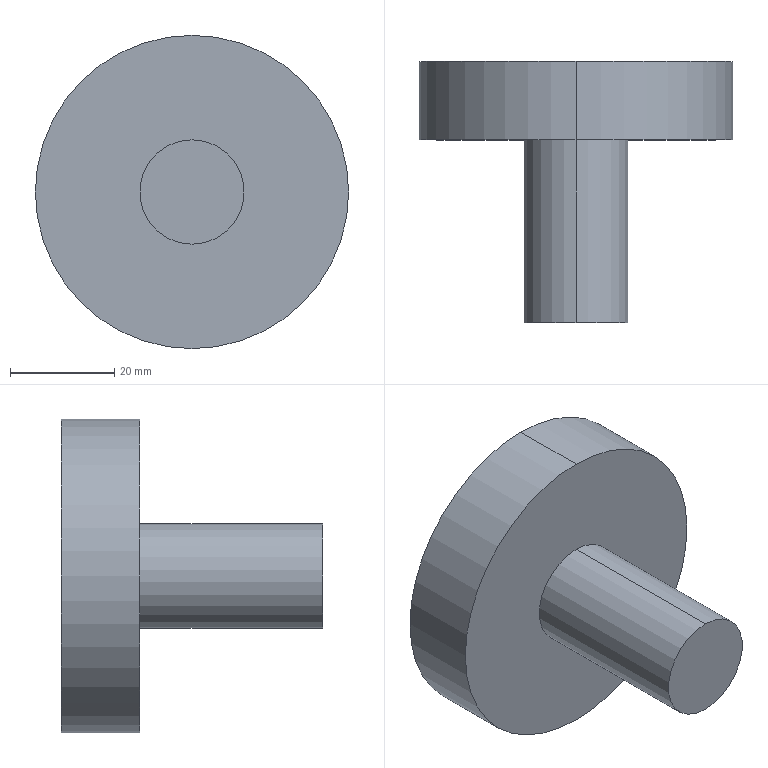Part | STEP file | Part5_1 | 1 solid | 16 faces | box 60 x 50 x 60 mm | volume 49793 mm3 | cylinder 10 | plane 6 | commonest cylinder face diameters 15.4 x2 16.4 x2 18.4 x2 20 x2 60 x2
STEP:
#1=CARTESIAN_POINT('',(0.,0.,0.));
#2=DIRECTION('',(0.,0.,1.));
#3=DIRECTION('',(1.,0.,0.));
#4=AXIS2_PLACEMENT_3D('',#1,#2,#3);
#5=CARTESIAN_POINT('',(0.,84.,-200.8));
#6=VERTEX_POINT('',#5);
#7=CARTESIAN_POINT('',(0.,99.,-200.8));
#8=VERTEX_POINT('',#7);
#9=CARTESIAN_POINT('',(0.,91.5,-200.8));
#10=DIRECTION('',(0.,1.,0.));
#11=VECTOR('',#10,1.);
#12=LINE('',#9,#11);
#13=CARTESIAN_POINT('',(0.,91.5,-210.));
#14=DIRECTION('',(0.,1.,0.));
#15=DIRECTION('',(0.,0.,1.));
#16=AXIS2_PLACEMENT_3D('',#13,#14,#15);
#17=CYLINDRICAL_SURFACE('',#16,9.2);
#18=CARTESIAN_POINT('',(6.283,0.));
#19=DIRECTION('',(0.,1.));
#20=VECTOR('',#19,1.);
#21=LINE('',#18,#20);
#22=(GEOMETRIC_REPRESENTATION_CONTEXT(2)PARAMETRIC_REPRESENTATION_CONTEXT()REPRESENTATION_CONTEXT('',''));
#23=DEFINITIONAL_REPRESENTATION('',(#21),#22);
#24=PCURVE('',#17,#23);
#25=CARTESIAN_POINT('',(0.,91.5,-210.));
#26=DIRECTION('',(0.,1.,0.));
#27=DIRECTION('',(0.,0.,1.));
#28=AXIS2_PLACEMENT_3D('',#25,#26,#27);
#29=CYLINDRICAL_SURFACE('',#28,9.2);
#30=CARTESIAN_POINT('',(0.,0.));
#31=DIRECTION('',(0.,1.));
#32=VECTOR('',#31,1.);
#33=LINE('',#30,#32);
#34=(GEOMETRIC_REPRESENTATION_CONTEXT(2)PARAMETRIC_REPRESENTATION_CONTEXT()REPRESENTATION_CONTEXT('',''));
#35=DEFINITIONAL_REPRESENTATION('',(#33),#34);
#36=PCURVE('',#29,#35);
#37=SURFACE_CURVE('',#12,(#24,#36),.PCURVE_S1.);
#38=EDGE_CURVE('',#6,#8,#37,.T.);
#39=ORIENTED_EDGE('',*,*,#38,.T.);
#40=CARTESIAN_POINT('',(0.,99.,-219.2));
#41=VERTEX_POINT('',#40);
#42=CARTESIAN_POINT('',(0.,99.,-210.));
#43=DIRECTION('',(0.,-1.,0.));
#44=DIRECTION('',(0.,0.,1.));
#45=AXIS2_PLACEMENT_3D('',#42,#43,#44);
#46=CIRCLE('',#45,9.2);
#47=CARTESIAN_POINT('',(6.283,7.5));
#48=DIRECTION('',(-1.,0.));
#49=VECTOR('',#48,1.);
#50=LINE('',#47,#49);
#51=(GEOMETRIC_REPRESENTATION_CONTEXT(2)PARAMETRIC_REPRESENTATION_CONTEXT()REPRESENTATION_CONTEXT('',''));
#52=DEFINITIONAL_REPRESENTATION('',(#50),#51);
#53=PCURVE('',#17,#52);
#54=CARTESIAN_POINT('',(0.,99.,0.));
#55=DIRECTION('',(0.,1.,0.));
#56=DIRECTION('',(0.,0.,1.));
#57=AXIS2_PLACEMENT_3D('',#54,#55,#56);
#58=PLANE('',#57);
#59=CARTESIAN_POINT('',(-200.8,0.));
#60=CARTESIAN_POINT('',(-200.8,-15.935));
#61=CARTESIAN_POINT('',(-214.6,-7.967));
#62=CARTESIAN_POINT('',(-228.4,0.));
#63=CARTESIAN_POINT('',(-214.6,7.967));
#64=CARTESIAN_POINT('',(-200.8,15.935));
#65=CARTESIAN_POINT('',(-200.8,0.));
#66=(BOUNDED_CURVE()B_SPLINE_CURVE(2,(#59,#60,#61,#62,#63,#64,#65),.UNSPECIFIED.,.T.,.F.)B_SPLINE_CURVE_WITH_KNOTS((1,2,2,2,2,1),(-2.094,0.,2.094,4.189,6.283,8.378),.UNSPECIFIED.)CURVE()GEOMETRIC_REPRESENTATION_ITEM()RATIONAL_B_SPLINE_CURVE((1.,0.5,1.,0.5,1.,0.5,1.))REPRESENTATION_ITEM(''));
#67=(GEOMETRIC_REPRESENTATION_CONTEXT(2)PARAMETRIC_REPRESENTATION_CONTEXT()REPRESENTATION_CONTEXT('',''));
#68=DEFINITIONAL_REPRESENTATION('',(#66),#67);
#69=PCURVE('',#58,#68);
#70=SURFACE_CURVE('',#46,(#53,#69),.PCURVE_S1.);
#71=EDGE_CURVE('',#8,#41,#70,.T.);
#72=ORIENTED_EDGE('',*,*,#71,.T.);
#73=CARTESIAN_POINT('',(0.,84.,-219.2));
#74=VERTEX_POINT('',#73);
#75=CARTESIAN_POINT('',(0.,91.5,-219.2));
#76=DIRECTION('',(0.,1.,0.));
#77=VECTOR('',#76,1.);
#78=LINE('',#75,#77);
#79=CARTESIAN_POINT('',(3.142,0.));
#80=DIRECTION('',(0.,1.));
#81=VECTOR('',#80,1.);
#82=LINE('',#79,#81);
#83=(GEOMETRIC_REPRESENTATION_CONTEXT(2)PARAMETRIC_REPRESENTATION_CONTEXT()REPRESENTATION_CONTEXT('',''));
#84=DEFINITIONAL_REPRESENTATION('',(#82),#83);
#85=PCURVE('',#17,#84);
#86=CARTESIAN_POINT('',(3.142,0.));
#87=DIRECTION('',(0.,1.));
#88=VECTOR('',#87,1.);
#89=LINE('',#86,#88);
#90=(GEOMETRIC_REPRESENTATION_CONTEXT(2)PARAMETRIC_REPRESENTATION_CONTEXT()REPRESENTATION_CONTEXT('',''));
#91=DEFINITIONAL_REPRESENTATION('',(#89),#90);
#92=PCURVE('',#29,#91);
#93=SURFACE_CURVE('',#78,(#85,#92),.PCURVE_S1.);
#94=EDGE_CURVE('',#74,#41,#93,.T.);
#95=ORIENTED_EDGE('',*,*,#94,.F.);
#96=CARTESIAN_POINT('',(0.,84.,-210.));
#97=DIRECTION('',(0.,1.,0.));
#98=DIRECTION('',(0.,0.,1.));
#99=AXIS2_PLACEMENT_3D('',#96,#97,#98);
#100=CIRCLE('',#99,9.2);
#101=CARTESIAN_POINT('',(0.,-7.5));
#102=DIRECTION('',(1.,0.));
#103=VECTOR('',#102,1.);
#104=LINE('',#101,#103);
#105=(GEOMETRIC_REPRESENTATION_CONTEXT(2)PARAMETRIC_REPRESENTATION_CONTEXT()REPRESENTATION_CONTEXT('',''));
#106=DEFINITIONAL_REPRESENTATION('',(#104),#105);
#107=PCURVE('',#17,#106);
#108=CARTESIAN_POINT('',(0.,84.,0.));
#109=DIRECTION('',(0.,1.,0.));
#110=DIRECTION('',(0.,0.,1.));
#111=AXIS2_PLACEMENT_3D('',#108,#109,#110);
#112=PLANE('',#111);
#113=CARTESIAN_POINT('',(-210.,0.));
#114=DIRECTION('',(1.,0.));
#115=AXIS2_PLACEMENT_2D('',#113,#114);
#116=CIRCLE('',#115,9.2);
#117=(GEOMETRIC_REPRESENTATION_CONTEXT(2)PARAMETRIC_REPRESENTATION_CONTEXT()REPRESENTATION_CONTEXT('',''));
#118=DEFINITIONAL_REPRESENTATION('',(#116),#117);
#119=PCURVE('',#112,#118);
#120=SURFACE_CURVE('',#100,(#107,#119),.PCURVE_S1.);
#121=EDGE_CURVE('',#74,#6,#120,.T.);
#122=ORIENTED_EDGE('',*,*,#121,.T.);
#123=EDGE_LOOP('',(#39,#72,#95,#122));
#124=FACE_BOUND('',#123,.F.);
#125=ADVANCED_FACE('',(#124),#17,.F.);
#126=CARTESIAN_POINT('',(0.,84.,-180.));
#127=VERTEX_POINT('',#126);
#128=CARTESIAN_POINT('',(0.,84.,-240.));
#129=VERTEX_POINT('',#128);
#130=CARTESIAN_POINT('',(0.,84.,-210.));
#131=DIRECTION('',(0.,1.,0.));
#132=DIRECTION('',(0.,0.,1.));
#133=AXIS2_PLACEMENT_3D('',#130,#131,#132);
#134=CIRCLE('',#133,30.);
#135=CARTESIAN_POINT('',(0.,91.5,-210.));
#136=DIRECTION('',(0.,1.,0.));
#137=DIRECTION('',(0.,0.,1.));
#138=AXIS2_PLACEMENT_3D('',#135,#136,#137);
#139=CYLINDRICAL_SURFACE('',#138,30.);
#140=CARTESIAN_POINT('',(0.,-7.5));
#141=DIRECTION('',(1.,0.));
#142=VECTOR('',#141,1.);
#143=LINE('',#140,#142);
#144=(GEOMETRIC_REPRESENTATION_CONTEXT(2)PARAMETRIC_REPRESENTATION_CONTEXT()REPRESENTATION_CONTEXT('',''));
#145=DEFINITIONAL_REPRESENTATION('',(#143),#144);
#146=PCURVE('',#139,#145);
#147=CARTESIAN_POINT('',(0.,84.,0.));
#148=DIRECTION('',(0.,1.,0.));
#149=DIRECTION('',(0.,0.,1.));
#150=AXIS2_PLACEMENT_3D('',#147,#148,#149);
#151=PLANE('',#150);
#152=CARTESIAN_POINT('',(-210.,0.));
#153=DIRECTION('',(1.,0.));
#154=AXIS2_PLACEMENT_2D('',#152,#153);
#155=CIRCLE('',#154,30.);
#156=(GEOMETRIC_REPRESENTATION_CONTEXT(2)PARAMETRIC_REPRESENTATION_CONTEXT()REPRESENTATION_CONTEXT('',''));
#157=DEFINITIONAL_REPRESENTATION('',(#155),#156);
#158=PCURVE('',#151,#157);
#159=SURFACE_CURVE('',#134,(#146,#158),.PCURVE_S1.);
#160=EDGE_CURVE('',#127,#129,#159,.T.);
#161=ORIENTED_EDGE('',*,*,#160,.T.);
#162=CARTESIAN_POINT('',(0.,99.,-240.));
#163=VERTEX_POINT('',#162);
#164=CARTESIAN_POINT('',(0.,91.5,-240.));
#165=DIRECTION('',(0.,1.,0.));
#166=VECTOR('',#165,1.);
#167=LINE('',#164,#166);
#168=CARTESIAN_POINT('',(3.142,0.));
#169=DIRECTION('',(0.,1.));
#170=VECTOR('',#169,1.);
#171=LINE('',#168,#170);
#172=(GEOMETRIC_REPRESENTATION_CONTEXT(2)PARAMETRIC_REPRESENTATION_CONTEXT()REPRESENTATION_CONTEXT('',''));
#173=DEFINITIONAL_REPRESENTATION('',(#171),#172);
#174=PCURVE('',#139,#173);
#175=CARTESIAN_POINT('',(0.,91.5,-210.));
#176=DIRECTION('',(0.,1.,0.));
#177=DIRECTION('',(0.,0.,1.));
#178=AXIS2_PLACEMENT_3D('',#175,#176,#177);
#179=CYLINDRICAL_SURFACE('',#178,30.);
#180=CARTESIAN_POINT('',(3.142,0.));
#181=DIRECTION('',(0.,1.));
#182=VECTOR('',#181,1.);
#183=LINE('',#180,#182);
#184=(GEOMETRIC_REPRESENTATION_CONTEXT(2)PARAMETRIC_REPRESENTATION_CONTEXT()REPRESENTATION_CONTEXT('',''));
#185=DEFINITIONAL_REPRESENTATION('',(#183),#184);
#186=PCURVE('',#179,#185);
#187=SURFACE_CURVE('',#167,(#174,#186),.PCURVE_S1.);
#188=EDGE_CURVE('',#129,#163,#187,.T.);
#189=ORIENTED_EDGE('',*,*,#188,.T.);
#190=CARTESIAN_POINT('',(0.,99.,-180.));
#191=VERTEX_POINT('',#190);
#192=CARTESIAN_POINT('',(0.,99.,-210.));
#193=DIRECTION('',(0.,1.,0.));
#194=DIRECTION('',(0.,0.,1.));
#195=AXIS2_PLACEMENT_3D('',#192,#193,#194);
#196=CIRCLE('',#195,30.);
#197=CARTESIAN_POINT('',(0.,7.5));
#198=DIRECTION('',(1.,0.));
#199=VECTOR('',#198,1.);
#200=LINE('',#197,#199);
#201=(GEOMETRIC_REPRESENTATION_CONTEXT(2)PARAMETRIC_REPRESENTATION_CONTEXT()REPRESENTATION_CONTEXT('',''));
#202=DEFINITIONAL_REPRESENTATION('',(#200),#201);
#203=PCURVE('',#139,#202);
#204=CARTESIAN_POINT('',(-210.,0.));
#205=DIRECTION('',(1.,0.));
#206=AXIS2_PLACEMENT_2D('',#204,#205);
#207=CIRCLE('',#206,30.);
#208=(GEOMETRIC_REPRESENTATION_CONTEXT(2)PARAMETRIC_REPRESENTATION_CONTEXT()REPRESENTATION_CONTEXT('',''));
#209=DEFINITIONAL_REPRESENTATION('',(#207),#208);
#210=PCURVE('',#58,#209);
#211=SURFACE_CURVE('',#196,(#203,#210),.PCURVE_S1.);
#212=EDGE_CURVE('',#191,#163,#211,.T.);
#213=ORIENTED_EDGE('',*,*,#212,.F.);
#214=CARTESIAN_POINT('',(0.,91.5,-180.));
#215=DIRECTION('',(0.,1.,0.));
#216=VECTOR('',#215,1.);
#217=LINE('',#214,#216);
#218=CARTESIAN_POINT('',(0.,0.));
#219=DIRECTION('',(0.,1.));
#220=VECTOR('',#219,1.);
#221=LINE('',#218,#220);
#222=(GEOMETRIC_REPRESENTATION_CONTEXT(2)PARAMETRIC_REPRESENTATION_CONTEXT()REPRESENTATION_CONTEXT('',''));
#223=DEFINITIONAL_REPRESENTATION('',(#221),#222);
#224=PCURVE('',#139,#223);
#225=CARTESIAN_POINT('',(6.283,0.));
#226=DIRECTION('',(0.,1.));
#227=VECTOR('',#226,1.);
#228=LINE('',#225,#227);
#229=(GEOMETRIC_REPRESENTATION_CONTEXT(2)PARAMETRIC_REPRESENTATION_CONTEXT()REPRESENTATION_CONTEXT('',''));
#230=DEFINITIONAL_REPRESENTATION('',(#228),#229);
#231=PCURVE('',#179,#230);
#232=SURFACE_CURVE('',#217,(#224,#231),.PCURVE_S1.);
#233=EDGE_CURVE('',#127,#191,#232,.T.);
#234=ORIENTED_EDGE('',*,*,#233,.F.);
#235=EDGE_LOOP('',(#161,#189,#213,#234));
#236=FACE_BOUND('',#235,.T.);
#237=ADVANCED_FACE('',(#236),#139,.T.);
#238=CARTESIAN_POINT('',(0.,84.,-218.2));
#239=VERTEX_POINT('',#238);
#240=CARTESIAN_POINT('',(0.,84.,-201.8));
#241=VERTEX_POINT('',#240);
#242=CARTESIAN_POINT('',(0.,84.,-210.));
#243=DIRECTION('',(0.,-1.,0.));
#244=DIRECTION('',(0.,0.,1.));
#245=AXIS2_PLACEMENT_3D('',#242,#243,#244);
#246=CIRCLE('',#245,8.2);
#247=CARTESIAN_POINT('',(0.,91.5,-210.));
#248=DIRECTION('',(0.,1.,0.));
#249=DIRECTION('',(0.,0.,1.));
#250=AXIS2_PLACEMENT_3D('',#247,#248,#249);
#251=CYLINDRICAL_SURFACE('',#250,8.2);
#252=CARTESIAN_POINT('',(6.283,-7.5));
#253=DIRECTION('',(-1.,0.));
#254=VECTOR('',#253,1.);
#255=LINE('',#252,#254);
#256=(GEOMETRIC_REPRESENTATION_CONTEXT(2)PARAMETRIC_REPRESENTATION_CONTEXT()REPRESENTATION_CONTEXT('',''));
#257=DEFINITIONAL_REPRESENTATION('',(#255),#256);
#258=PCURVE('',#251,#257);
#259=CARTESIAN_POINT('',(-201.8,0.));
#260=CARTESIAN_POINT('',(-201.8,-14.203));
#261=CARTESIAN_POINT('',(-214.1,-7.101));
#262=CARTESIAN_POINT('',(-226.4,0.));
#263=CARTESIAN_POINT('',(-214.1,7.101));
#264=CARTESIAN_POINT('',(-201.8,14.203));
#265=CARTESIAN_POINT('',(-201.8,0.));
#266=(BOUNDED_CURVE()B_SPLINE_CURVE(2,(#259,#260,#261,#262,#263,#264,#265),.UNSPECIFIED.,.T.,.F.)B_SPLINE_CURVE_WITH_KNOTS((1,2,2,2,2,1),(-2.094,0.,2.094,4.189,6.283,8.378),.UNSPECIFIED.)CURVE()GEOMETRIC_REPRESENTATION_ITEM()RATIONAL_B_SPLINE_CURVE((1.,0.5,1.,0.5,1.,0.5,1.))REPRESENTATION_ITEM(''));
#267=(GEOMETRIC_REPRESENTATION_CONTEXT(2)PARAMETRIC_REPRESENTATION_CONTEXT()REPRESENTATION_CONTEXT('',''));
#268=DEFINITIONAL_REPRESENTATION('',(#266),#267);
#269=PCURVE('',#112,#268);
#270=SURFACE_CURVE('',#246,(#258,#269),.PCURVE_S1.);
#271=EDGE_CURVE('',#239,#241,#270,.T.);
#272=ORIENTED_EDGE('',*,*,#271,.F.);
#273=CARTESIAN_POINT('',(0.,99.,-218.2));
#274=VERTEX_POINT('',#273);
#275=CARTESIAN_POINT('',(0.,91.5,-218.2));
#276=DIRECTION('',(0.,1.,0.));
#277=VECTOR('',#276,1.);
#278=LINE('',#275,#277);
#279=CARTESIAN_POINT('',(3.142,0.));
#280=DIRECTION('',(0.,1.));
#281=VECTOR('',#280,1.);
#282=LINE('',#279,#281);
#283=(GEOMETRIC_REPRESENTATION_CONTEXT(2)PARAMETRIC_REPRESENTATION_CONTEXT()REPRESENTATION_CONTEXT('',''));
#284=DEFINITIONAL_REPRESENTATION('',(#282),#283);
#285=PCURVE('',#251,#284);
#286=CARTESIAN_POINT('',(0.,91.5,-210.));
#287=DIRECTION('',(0.,1.,0.));
#288=DIRECTION('',(0.,0.,1.));
#289=AXIS2_PLACEMENT_3D('',#286,#287,#288);
#290=CYLINDRICAL_SURFACE('',#289,8.2);
#291=CARTESIAN_POINT('',(3.142,0.));
#292=DIRECTION('',(0.,1.));
#293=VECTOR('',#292,1.);
#294=LINE('',#291,#293);
#295=(GEOMETRIC_REPRESENTATION_CONTEXT(2)PARAMETRIC_REPRESENTATION_CONTEXT()REPRESENTATION_CONTEXT('',''));
#296=DEFINITIONAL_REPRESENTATION('',(#294),#295);
#297=PCURVE('',#290,#296);
#298=SURFACE_CURVE('',#278,(#285,#297),.PCURVE_S1.);
#299=EDGE_CURVE('',#239,#274,#298,.T.);
#300=ORIENTED_EDGE('',*,*,#299,.T.);
#301=CARTESIAN_POINT('',(0.,99.,-201.8));
#302=VERTEX_POINT('',#301);
#303=CARTESIAN_POINT('',(0.,99.,-210.));
#304=DIRECTION('',(0.,-1.,0.));
#305=DIRECTION('',(0.,0.,1.));
#306=AXIS2_PLACEMENT_3D('',#303,#304,#305);
#307=CIRCLE('',#306,8.2);
#308=CARTESIAN_POINT('',(6.283,7.5));
#309=DIRECTION('',(-1.,0.));
#310=VECTOR('',#309,1.);
#311=LINE('',#308,#310);
#312=(GEOMETRIC_REPRESENTATION_CONTEXT(2)PARAMETRIC_REPRESENTATION_CONTEXT()REPRESENTATION_CONTEXT('',''));
#313=DEFINITIONAL_REPRESENTATION('',(#311),#312);
#314=PCURVE('',#251,#313);
#315=CARTESIAN_POINT('',(0.,99.,0.));
#316=DIRECTION('',(0.,1.,0.));
#317=DIRECTION('',(0.,0.,1.));
#318=AXIS2_PLACEMENT_3D('',#315,#316,#317);
#319=PLANE('',#318);
#320=CARTESIAN_POINT('',(-201.8,0.));
#321=CARTESIAN_POINT('',(-201.8,-14.203));
#322=CARTESIAN_POINT('',(-214.1,-7.101));
#323=CARTESIAN_POINT('',(-226.4,0.));
#324=CARTESIAN_POINT('',(-214.1,7.101));
#325=CARTESIAN_POINT('',(-201.8,14.203));
#326=CARTESIAN_POINT('',(-201.8,0.));
#327=(BOUNDED_CURVE()B_SPLINE_CURVE(2,(#320,#321,#322,#323,#324,#325,#326),.UNSPECIFIED.,.T.,.F.)B_SPLINE_CURVE_WITH_KNOTS((1,2,2,2,2,1),(-2.094,0.,2.094,4.189,6.283,8.378),.UNSPECIFIED.)CURVE()GEOMETRIC_REPRESENTATION_ITEM()RATIONAL_B_SPLINE_CURVE((1.,0.5,1.,0.5,1.,0.5,1.))REPRESENTATION_ITEM(''));
#328=(GEOMETRIC_REPRESENTATION_CONTEXT(2)PARAMETRIC_REPRESENTATION_CONTEXT()REPRESENTATION_CONTEXT('',''));
#329=DEFINITIONAL_REPRESENTATION('',(#327),#328);
#330=PCURVE('',#319,#329);
#331=SURFACE_CURVE('',#307,(#314,#330),.PCURVE_S1.);
#332=EDGE_CURVE('',#274,#302,#331,.T.);
#333=ORIENTED_EDGE('',*,*,#332,.T.);
#334=CARTESIAN_POINT('',(0.,91.5,-201.8));
#335=DIRECTION('',(0.,1.,0.));
#336=VECTOR('',#335,1.);
#337=LINE('',#334,#336);
#338=CARTESIAN_POINT('',(0.,0.));
#339=DIRECTION('',(0.,1.));
#340=VECTOR('',#339,1.);
#341=LINE('',#338,#340);
#342=(GEOMETRIC_REPRESENTATION_CONTEXT(2)PARAMETRIC_REPRESENTATION_CONTEXT()REPRESENTATION_CONTEXT('',''));
#343=DEFINITIONAL_REPRESENTATION('',(#341),#342);
#344=PCURVE('',#251,#343);
#345=CARTESIAN_POINT('',(6.283,0.));
#346=DIRECTION('',(0.,1.));
#347=VECTOR('',#346,1.);
#348=LINE('',#345,#347);
#349=(GEOMETRIC_REPRESENTATION_CONTEXT(2)PARAMETRIC_REPRESENTATION_CONTEXT()REPRESENTATION_CONTEXT('',''));
#350=DEFINITIONAL_REPRESENTATION('',(#348),#349);
#351=PCURVE('',#290,#350);
#352=SURFACE_CURVE('',#337,(#344,#351),.PCURVE_S1.);
#353=EDGE_CURVE('',#241,#302,#352,.T.);
#354=ORIENTED_EDGE('',*,*,#353,.F.);
#355=EDGE_LOOP('',(#272,#300,#333,#354));
#356=FACE_BOUND('',#355,.T.);
#357=ADVANCED_FACE('',(#356),#251,.T.);
#358=CARTESIAN_POINT('',(0.,49.,-200.));
#359=VERTEX_POINT('',#358);
#360=CARTESIAN_POINT('',(0.,49.,-220.));
#361=VERTEX_POINT('',#360);
#362=CARTESIAN_POINT('',(0.,49.,-210.));
#363=DIRECTION('',(0.,1.,0.));
#364=DIRECTION('',(0.,0.,1.));
#365=AXIS2_PLACEMENT_3D('',#362,#363,#364);
#366=CIRCLE('',#365,10.);
#367=CARTESIAN_POINT('',(0.,66.5,-210.));
#368=DIRECTION('',(0.,1.,0.));
#369=DIRECTION('',(0.,0.,1.));
#370=AXIS2_PLACEMENT_3D('',#367,#368,#369);
#371=CYLINDRICAL_SURFACE('',#370,10.);
#372=CARTESIAN_POINT('',(0.,-17.5));
#373=DIRECTION('',(1.,0.));
#374=VECTOR('',#373,1.);
#375=LINE('',#372,#374);
#376=(GEOMETRIC_REPRESENTATION_CONTEXT(2)PARAMETRIC_REPRESENTATION_CONTEXT()REPRESENTATION_CONTEXT('',''));
#377=DEFINITIONAL_REPRESENTATION('',(#375),#376);
#378=PCURVE('',#371,#377);
#379=CARTESIAN_POINT('',(0.,49.,0.));
#380=DIRECTION('',(0.,1.,0.));
#381=DIRECTION('',(0.,0.,1.));
#382=AXIS2_PLACEMENT_3D('',#379,#380,#381);
#383=PLANE('',#382);
#384=CARTESIAN_POINT('',(-210.,0.));
#385=DIRECTION('',(1.,0.));
#386=AXIS2_PLACEMENT_2D('',#384,#385);
#387=CIRCLE('',#386,10.);
#388=(GEOMETRIC_REPRESENTATION_CONTEXT(2)PARAMETRIC_REPRESENTATION_CONTEXT()REPRESENTATION_CONTEXT('',''));
#389=DEFINITIONAL_REPRESENTATION('',(#387),#388);
#390=PCURVE('',#383,#389);
#391=SURFACE_CURVE('',#366,(#378,#390),.PCURVE_S1.);
#392=EDGE_CURVE('',#359,#361,#391,.T.);
#393=ORIENTED_EDGE('',*,*,#392,.T.);
#394=CARTESIAN_POINT('',(0.,84.,-220.));
#395=VERTEX_POINT('',#394);
#396=CARTESIAN_POINT('',(0.,66.5,-220.));
#397=DIRECTION('',(0.,1.,0.));
#398=VECTOR('',#397,1.);
#399=LINE('',#396,#398);
#400=CARTESIAN_POINT('',(3.142,0.));
#401=DIRECTION('',(0.,1.));
#402=VECTOR('',#401,1.);
#403=LINE('',#400,#402);
#404=(GEOMETRIC_REPRESENTATION_CONTEXT(2)PARAMETRIC_REPRESENTATION_CONTEXT()REPRESENTATION_CONTEXT('',''));
#405=DEFINITIONAL_REPRESENTATION('',(#403),#404);
#406=PCURVE('',#371,#405);
#407=CARTESIAN_POINT('',(0.,66.5,-210.));
#408=DIRECTION('',(0.,1.,0.));
#409=DIRECTION('',(0.,0.,1.));
#410=AXIS2_PLACEMENT_3D('',#407,#408,#409);
#411=CYLINDRICAL_SURFACE('',#410,10.);
#412=CARTESIAN_POINT('',(3.142,0.));
#413=DIRECTION('',(0.,1.));
#414=VECTOR('',#413,1.);
#415=LINE('',#412,#414);
#416=(GEOMETRIC_REPRESENTATION_CONTEXT(2)PARAMETRIC_REPRESENTATION_CONTEXT()REPRESENTATION_CONTEXT('',''));
#417=DEFINITIONAL_REPRESENTATION('',(#415),#416);
#418=PCURVE('',#411,#417);
#419=SURFACE_CURVE('',#399,(#406,#418),.PCURVE_S1.);
#420=EDGE_CURVE('',#361,#395,#419,.T.);
#421=ORIENTED_EDGE('',*,*,#420,.T.);
#422=CARTESIAN_POINT('',(0.,84.,-200.));
#423=VERTEX_POINT('',#422);
#424=CARTESIAN_POINT('',(0.,84.,-210.));
#425=DIRECTION('',(0.,-1.,0.));
#426=DIRECTION('',(0.,0.,1.));
#427=AXIS2_PLACEMENT_3D('',#424,#425,#426);
#428=CIRCLE('',#427,10.);
#429=CARTESIAN_POINT('',(6.283,17.5));
#430=DIRECTION('',(-1.,0.));
#431=VECTOR('',#430,1.);
#432=LINE('',#429,#431);
#433=(GEOMETRIC_REPRESENTATION_CONTEXT(2)PARAMETRIC_REPRESENTATION_CONTEXT()REPRESENTATION_CONTEXT('',''));
#434=DEFINITIONAL_REPRESENTATION('',(#432),#433);
#435=PCURVE('',#371,#434);
#436=CARTESIAN_POINT('',(-200.,0.));
#437=CARTESIAN_POINT('',(-200.,-17.321));
#438=CARTESIAN_POINT('',(-215.,-8.66));
#439=CARTESIAN_POINT('',(-230.,0.));
#440=CARTESIAN_POINT('',(-215.,8.66));
#441=CARTESIAN_POINT('',(-200.,17.321));
#442=CARTESIAN_POINT('',(-200.,0.));
#443=(BOUNDED_CURVE()B_SPLINE_CURVE(2,(#436,#437,#438,#439,#440,#441,#442),.UNSPECIFIED.,.T.,.F.)B_SPLINE_CURVE_WITH_KNOTS((1,2,2,2,2,1),(-2.094,0.,2.094,4.189,6.283,8.378),.UNSPECIFIED.)CURVE()GEOMETRIC_REPRESENTATION_ITEM()RATIONAL_B_SPLINE_CURVE((1.,0.5,1.,0.5,1.,0.5,1.))REPRESENTATION_ITEM(''));
#444=(GEOMETRIC_REPRESENTATION_CONTEXT(2)PARAMETRIC_REPRESENTATION_CONTEXT()REPRESENTATION_CONTEXT('',''));
#445=DEFINITIONAL_REPRESENTATION('',(#443),#444);
#446=PCURVE('',#151,#445);
#447=SURFACE_CURVE('',#428,(#435,#446),.PCURVE_S1.);
#448=EDGE_CURVE('',#395,#423,#447,.T.);
#449=ORIENTED_EDGE('',*,*,#448,.T.);
#450=CARTESIAN_POINT('',(0.,66.5,-200.));
#451=DIRECTION('',(0.,1.,0.));
#452=VECTOR('',#451,1.);
#453=LINE('',#450,#452);
#454=CARTESIAN_POINT('',(0.,0.));
#455=DIRECTION('',(0.,1.));
#456=VECTOR('',#455,1.);
#457=LINE('',#454,#456);
#458=(GEOMETRIC_REPRESENTATION_CONTEXT(2)PARAMETRIC_REPRESENTATION_CONTEXT()REPRESENTATION_CONTEXT('',''));
#459=DEFINITIONAL_REPRESENTATION('',(#457),#458);
#460=PCURVE('',#371,#459);
#461=CARTESIAN_POINT('',(6.283,0.));
#462=DIRECTION('',(0.,1.));
#463=VECTOR('',#462,1.);
#464=LINE('',#461,#463);
#465=(GEOMETRIC_REPRESENTATION_CONTEXT(2)PARAMETRIC_REPRESENTATION_CONTEXT()REPRESENTATION_CONTEXT('',''));
#466=DEFINITIONAL_REPRESENTATION('',(#464),#465);
#467=PCURVE('',#411,#466);
#468=SURFACE_CURVE('',#453,(#460,#467),.PCURVE_S1.);
#469=EDGE_CURVE('',#359,#423,#468,.T.);
#470=ORIENTED_EDGE('',*,*,#469,.F.);
#471=EDGE_LOOP('',(#393,#421,#449,#470));
#472=FACE_BOUND('',#471,.T.);
#473=ADVANCED_FACE('',(#472),#371,.T.);
#474=CARTESIAN_POINT('',(0.,84.,-202.3));
#475=VERTEX_POINT('',#474);
#476=CARTESIAN_POINT('',(0.,99.,-202.3));
#477=VERTEX_POINT('',#476);
#478=CARTESIAN_POINT('',(0.,91.5,-202.3));
#479=DIRECTION('',(0.,1.,0.));
#480=VECTOR('',#479,1.);
#481=LINE('',#478,#480);
#482=CARTESIAN_POINT('',(0.,91.5,-210.));
#483=DIRECTION('',(0.,1.,0.));
#484=DIRECTION('',(0.,0.,1.));
#485=AXIS2_PLACEMENT_3D('',#482,#483,#484);
#486=CYLINDRICAL_SURFACE('',#485,7.7);
#487=CARTESIAN_POINT('',(6.283,0.));
#488=DIRECTION('',(0.,1.));
#489=VECTOR('',#488,1.);
#490=LINE('',#487,#489);
#491=(GEOMETRIC_REPRESENTATION_CONTEXT(2)PARAMETRIC_REPRESENTATION_CONTEXT()REPRESENTATION_CONTEXT('',''));
#492=DEFINITIONAL_REPRESENTATION('',(#490),#491);
#493=PCURVE('',#486,#492);
#494=CARTESIAN_POINT('',(0.,91.5,-210.));
#495=DIRECTION('',(0.,1.,0.));
#496=DIRECTION('',(0.,0.,1.));
#497=AXIS2_PLACEMENT_3D('',#494,#495,#496);
#498=CYLINDRICAL_SURFACE('',#497,7.7);
#499=CARTESIAN_POINT('',(0.,0.));
#500=DIRECTION('',(0.,1.));
#501=VECTOR('',#500,1.);
#502=LINE('',#499,#501);
#503=(GEOMETRIC_REPRESENTATION_CONTEXT(2)PARAMETRIC_REPRESENTATION_CONTEXT()REPRESENTATION_CONTEXT('',''));
#504=DEFINITIONAL_REPRESENTATION('',(#502),#503);
#505=PCURVE('',#498,#504);
#506=SURFACE_CURVE('',#481,(#493,#505),.PCURVE_S1.);
#507=EDGE_CURVE('',#475,#477,#506,.T.);
#508=ORIENTED_EDGE('',*,*,#507,.T.);
#509=CARTESIAN_POINT('',(0.,99.,-217.7));
#510=VERTEX_POINT('',#509);
#511=CARTESIAN_POINT('',(0.,99.,-210.));
#512=DIRECTION('',(0.,-1.,0.));
#513=DIRECTION('',(0.,0.,1.));
#514=AXIS2_PLACEMENT_3D('',#511,#512,#513);
#515=CIRCLE('',#514,7.7);
#516=CARTESIAN_POINT('',(6.283,7.5));
#517=DIRECTION('',(-1.,0.));
#518=VECTOR('',#517,1.);
#519=LINE('',#516,#518);
#520=(GEOMETRIC_REPRESENTATION_CONTEXT(2)PARAMETRIC_REPRESENTATION_CONTEXT()REPRESENTATION_CONTEXT('',''));
#521=DEFINITIONAL_REPRESENTATION('',(#519),#520);
#522=PCURVE('',#486,#521);
#523=CARTESIAN_POINT('',(-202.3,0.));
#524=CARTESIAN_POINT('',(-202.3,-13.337));
#525=CARTESIAN_POINT('',(-213.85,-6.668));
#526=CARTESIAN_POINT('',(-225.4,0.));
#527=CARTESIAN_POINT('',(-213.85,6.668));
#528=CARTESIAN_POINT('',(-202.3,13.337));
#529=CARTESIAN_POINT('',(-202.3,0.));
#530=(BOUNDED_CURVE()B_SPLINE_CURVE(2,(#523,#524,#525,#526,#527,#528,#529),.UNSPECIFIED.,.T.,.F.)B_SPLINE_CURVE_WITH_KNOTS((1,2,2,2,2,1),(-2.094,0.,2.094,4.189,6.283,8.378),.UNSPECIFIED.)CURVE()GEOMETRIC_REPRESENTATION_ITEM()RATIONAL_B_SPLINE_CURVE((1.,0.5,1.,0.5,1.,0.5,1.))REPRESENTATION_ITEM(''));
#531=(GEOMETRIC_REPRESENTATION_CONTEXT(2)PARAMETRIC_REPRESENTATION_CONTEXT()REPRESENTATION_CONTEXT('',''));
#532=DEFINITIONAL_REPRESENTATION('',(#530),#531);
#533=PCURVE('',#319,#532);
#534=SURFACE_CURVE('',#515,(#522,#533),.PCURVE_S1.);
#535=EDGE_CURVE('',#477,#510,#534,.T.);
#536=ORIENTED_EDGE('',*,*,#535,.T.);
#537=CARTESIAN_POINT('',(0.,84.,-217.7));
#538=VERTEX_POINT('',#537);
#539=CARTESIAN_POINT('',(0.,91.5,-217.7));
#540=DIRECTION('',(0.,1.,0.));
#541=VECTOR('',#540,1.);
#542=LINE('',#539,#541);
#543=CARTESIAN_POINT('',(3.142,0.));
#544=DIRECTION('',(0.,1.));
#545=VECTOR('',#544,1.);
#546=LINE('',#543,#545);
#547=(GEOMETRIC_REPRESENTATION_CONTEXT(2)PARAMETRIC_REPRESENTATION_CONTEXT()REPRESENTATION_CONTEXT('',''));
#548=DEFINITIONAL_REPRESENTATION('',(#546),#547);
#549=PCURVE('',#486,#548);
#550=CARTESIAN_POINT('',(3.142,0.));
#551=DIRECTION('',(0.,1.));
#552=VECTOR('',#551,1.);
#553=LINE('',#550,#552);
#554=(GEOMETRIC_REPRESENTATION_CONTEXT(2)PARAMETRIC_REPRESENTATION_CONTEXT()REPRESENTATION_CONTEXT('',''));
#555=DEFINITIONAL_REPRESENTATION('',(#553),#554);
#556=PCURVE('',#498,#555);
#557=SURFACE_CURVE('',#542,(#549,#556),.PCURVE_S1.);
#558=EDGE_CURVE('',#538,#510,#557,.T.);
#559=ORIENTED_EDGE('',*,*,#558,.F.);
#560=CARTESIAN_POINT('',(0.,84.,-210.));
#561=DIRECTION('',(0.,1.,0.));
#562=DIRECTION('',(0.,0.,1.));
#563=AXIS2_PLACEMENT_3D('',#560,#561,#562);
#564=CIRCLE('',#563,7.7);
#565=CARTESIAN_POINT('',(0.,-7.5));
#566=DIRECTION('',(1.,0.));
#567=VECTOR('',#566,1.);
#568=LINE('',#565,#567);
#569=(GEOMETRIC_REPRESENTATION_CONTEXT(2)PARAMETRIC_REPRESENTATION_CONTEXT()REPRESENTATION_CONTEXT('',''));
#570=DEFINITIONAL_REPRESENTATION('',(#568),#569);
#571=PCURVE('',#486,#570);
#572=CARTESIAN_POINT('',(0.,84.,0.));
#573=DIRECTION('',(0.,1.,0.));
#574=DIRECTION('',(0.,0.,1.));
#575=AXIS2_PLACEMENT_3D('',#572,#573,#574);
#576=PLANE('',#575);
#577=CARTESIAN_POINT('',(-210.,0.));
#578=DIRECTION('',(1.,0.));
#579=AXIS2_PLACEMENT_2D('',#577,#578);
#580=CIRCLE('',#579,7.7);
#581=(GEOMETRIC_REPRESENTATION_CONTEXT(2)PARAMETRIC_REPRESENTATION_CONTEXT()REPRESENTATION_CONTEXT('',''));
#582=DEFINITIONAL_REPRESENTATION('',(#580),#581);
#583=PCURVE('',#576,#582);
#584=SURFACE_CURVE('',#564,(#571,#583),.PCURVE_S1.);
#585=EDGE_CURVE('',#538,#475,#584,.T.);
#586=ORIENTED_EDGE('',*,*,#585,.T.);
#587=EDGE_LOOP('',(#508,#536,#559,#586));
#588=FACE_BOUND('',#587,.F.);
#589=ADVANCED_FACE('',(#588),#486,.F.);
#590=CARTESIAN_POINT('',(0.,84.,-210.));
#591=DIRECTION('',(0.,1.,0.));
#592=DIRECTION('',(0.,0.,1.));
#593=AXIS2_PLACEMENT_3D('',#590,#591,#592);
#594=CIRCLE('',#593,7.7);
#595=CARTESIAN_POINT('',(-210.,0.));
#596=DIRECTION('',(1.,0.));
#597=AXIS2_PLACEMENT_2D('',#595,#596);
#598=CIRCLE('',#597,7.7);
#599=(GEOMETRIC_REPRESENTATION_CONTEXT(2)PARAMETRIC_REPRESENTATION_CONTEXT()REPRESENTATION_CONTEXT('',''));
#600=DEFINITIONAL_REPRESENTATION('',(#598),#599);
#601=PCURVE('',#576,#600);
#602=CARTESIAN_POINT('',(0.,-7.5));
#603=DIRECTION('',(1.,0.));
#604=VECTOR('',#603,1.);
#605=LINE('',#602,#604);
#606=(GEOMETRIC_REPRESENTATION_CONTEXT(2)PARAMETRIC_REPRESENTATION_CONTEXT()REPRESENTATION_CONTEXT('',''));
#607=DEFINITIONAL_REPRESENTATION('',(#605),#606);
#608=PCURVE('',#498,#607);
#609=SURFACE_CURVE('',#594,(#601,#608),.PCURVE_S1.);
#610=EDGE_CURVE('',#475,#538,#609,.T.);
#611=ORIENTED_EDGE('',*,*,#610,.T.);
#612=ORIENTED_EDGE('',*,*,#585,.T.);
#613=EDGE_LOOP('',(#611,#612));
#614=FACE_BOUND('',#613,.T.);
#615=ADVANCED_FACE('',(#614),#576,.T.);
#616=CARTESIAN_POINT('',(0.,99.,-210.));
#617=DIRECTION('',(0.,-1.,0.));
#618=DIRECTION('',(0.,0.,1.));
#619=AXIS2_PLACEMENT_3D('',#616,#617,#618);
#620=CIRCLE('',#619,7.7);
#621=CARTESIAN_POINT('',(6.283,7.5));
#622=DIRECTION('',(-1.,0.));
#623=VECTOR('',#622,1.);
#624=LINE('',#621,#623);
#625=(GEOMETRIC_REPRESENTATION_CONTEXT(2)PARAMETRIC_REPRESENTATION_CONTEXT()REPRESENTATION_CONTEXT('',''));
#626=DEFINITIONAL_REPRESENTATION('',(#624),#625);
#627=PCURVE('',#498,#626);
#628=CARTESIAN_POINT('',(-202.3,0.));
#629=CARTESIAN_POINT('',(-202.3,-13.337));
#630=CARTESIAN_POINT('',(-213.85,-6.668));
#631=CARTESIAN_POINT('',(-225.4,0.));
#632=CARTESIAN_POINT('',(-213.85,6.668));
#633=CARTESIAN_POINT('',(-202.3,13.337));
#634=CARTESIAN_POINT('',(-202.3,0.));
#635=(BOUNDED_CURVE()B_SPLINE_CURVE(2,(#628,#629,#630,#631,#632,#633,#634),.UNSPECIFIED.,.T.,.F.)B_SPLINE_CURVE_WITH_KNOTS((1,2,2,2,2,1),(-2.094,0.,2.094,4.189,6.283,8.378),.UNSPECIFIED.)CURVE()GEOMETRIC_REPRESENTATION_ITEM()RATIONAL_B_SPLINE_CURVE((1.,0.5,1.,0.5,1.,0.5,1.))REPRESENTATION_ITEM(''));
#636=(GEOMETRIC_REPRESENTATION_CONTEXT(2)PARAMETRIC_REPRESENTATION_CONTEXT()REPRESENTATION_CONTEXT('',''));
#637=DEFINITIONAL_REPRESENTATION('',(#635),#636);
#638=PCURVE('',#319,#637);
#639=SURFACE_CURVE('',#620,(#627,#638),.PCURVE_S1.);
#640=EDGE_CURVE('',#510,#477,#639,.T.);
#641=ORIENTED_EDGE('',*,*,#640,.T.);
#642=ORIENTED_EDGE('',*,*,#507,.F.);
#643=ORIENTED_EDGE('',*,*,#610,.T.);
#644=ORIENTED_EDGE('',*,*,#558,.T.);
#645=EDGE_LOOP('',(#641,#642,#643,#644));
#646=FACE_BOUND('',#645,.F.);
#647=ADVANCED_FACE('',(#646),#498,.F.);
#648=ORIENTED_EDGE('',*,*,#392,.F.);
#649=CARTESIAN_POINT('',(0.,49.,-210.));
#650=DIRECTION('',(0.,1.,0.));
#651=DIRECTION('',(0.,0.,1.));
#652=AXIS2_PLACEMENT_3D('',#649,#650,#651);
#653=CIRCLE('',#652,10.);
#654=CARTESIAN_POINT('',(-210.,0.));
#655=DIRECTION('',(1.,0.));
#656=AXIS2_PLACEMENT_2D('',#654,#655);
#657=CIRCLE('',#656,10.);
#658=(GEOMETRIC_REPRESENTATION_CONTEXT(2)PARAMETRIC_REPRESENTATION_CONTEXT()REPRESENTATION_CONTEXT('',''));
#659=DEFINITIONAL_REPRESENTATION('',(#657),#658);
#660=PCURVE('',#383,#659);
#661=CARTESIAN_POINT('',(0.,-17.5));
#662=DIRECTION('',(1.,0.));
#663=VECTOR('',#662,1.);
#664=LINE('',#661,#663);
#665=(GEOMETRIC_REPRESENTATION_CONTEXT(2)PARAMETRIC_REPRESENTATION_CONTEXT()REPRESENTATION_CONTEXT('',''));
#666=DEFINITIONAL_REPRESENTATION('',(#664),#665);
#667=PCURVE('',#411,#666);
#668=SURFACE_CURVE('',#653,(#660,#667),.PCURVE_S1.);
#669=EDGE_CURVE('',#361,#359,#668,.T.);
#670=ORIENTED_EDGE('',*,*,#669,.F.);
#671=EDGE_LOOP('',(#648,#670));
#672=FACE_BOUND('',#671,.T.);
#673=ADVANCED_FACE('',(#672),#383,.F.);
#674=ORIENTED_EDGE('',*,*,#535,.T.);
#675=ORIENTED_EDGE('',*,*,#640,.T.);
#676=EDGE_LOOP('',(#674,#675));
#677=FACE_BOUND('',#676,.T.);
#678=CARTESIAN_POINT('',(0.,99.,-210.));
#679=DIRECTION('',(0.,-1.,0.));
#680=DIRECTION('',(0.,0.,1.));
#681=AXIS2_PLACEMENT_3D('',#678,#679,#680);
#682=CIRCLE('',#681,8.2);
#683=CARTESIAN_POINT('',(-201.8,0.));
#684=CARTESIAN_POINT('',(-201.8,-14.203));
#685=CARTESIAN_POINT('',(-214.1,-7.101));
#686=CARTESIAN_POINT('',(-226.4,0.));
#687=CARTESIAN_POINT('',(-214.1,7.101));
#688=CARTESIAN_POINT('',(-201.8,14.203));
#689=CARTESIAN_POINT('',(-201.8,0.));
#690=(BOUNDED_CURVE()B_SPLINE_CURVE(2,(#683,#684,#685,#686,#687,#688,#689),.UNSPECIFIED.,.T.,.F.)B_SPLINE_CURVE_WITH_KNOTS((1,2,2,2,2,1),(-2.094,0.,2.094,4.189,6.283,8.378),.UNSPECIFIED.)CURVE()GEOMETRIC_REPRESENTATION_ITEM()RATIONAL_B_SPLINE_CURVE((1.,0.5,1.,0.5,1.,0.5,1.))REPRESENTATION_ITEM(''));
#691=(GEOMETRIC_REPRESENTATION_CONTEXT(2)PARAMETRIC_REPRESENTATION_CONTEXT()REPRESENTATION_CONTEXT('',''));
#692=DEFINITIONAL_REPRESENTATION('',(#690),#691);
#693=PCURVE('',#319,#692);
#694=CARTESIAN_POINT('',(6.283,7.5));
#695=DIRECTION('',(-1.,0.));
#696=VECTOR('',#695,1.);
#697=LINE('',#694,#696);
#698=(GEOMETRIC_REPRESENTATION_CONTEXT(2)PARAMETRIC_REPRESENTATION_CONTEXT()REPRESENTATION_CONTEXT('',''));
#699=DEFINITIONAL_REPRESENTATION('',(#697),#698);
#700=PCURVE('',#290,#699);
#701=SURFACE_CURVE('',#682,(#693,#700),.PCURVE_S1.);
#702=EDGE_CURVE('',#302,#274,#701,.T.);
#703=ORIENTED_EDGE('',*,*,#702,.F.);
#704=ORIENTED_EDGE('',*,*,#332,.F.);
#705=EDGE_LOOP('',(#703,#704));
#706=FACE_BOUND('',#705,.T.);
#707=ADVANCED_FACE('',(#677,#706),#319,.T.);
#708=ORIENTED_EDGE('',*,*,#420,.F.);
#709=ORIENTED_EDGE('',*,*,#669,.T.);
#710=ORIENTED_EDGE('',*,*,#469,.T.);
#711=CARTESIAN_POINT('',(0.,84.,-210.));
#712=DIRECTION('',(0.,-1.,0.));
#713=DIRECTION('',(0.,0.,1.));
#714=AXIS2_PLACEMENT_3D('',#711,#712,#713);
#715=CIRCLE('',#714,10.);
#716=CARTESIAN_POINT('',(6.283,17.5));
#717=DIRECTION('',(-1.,0.));
#718=VECTOR('',#717,1.);
#719=LINE('',#716,#718);
#720=(GEOMETRIC_REPRESENTATION_CONTEXT(2)PARAMETRIC_REPRESENTATION_CONTEXT()REPRESENTATION_CONTEXT('',''));
#721=DEFINITIONAL_REPRESENTATION('',(#719),#720);
#722=PCURVE('',#411,#721);
#723=CARTESIAN_POINT('',(-200.,0.));
#724=CARTESIAN_POINT('',(-200.,-17.321));
#725=CARTESIAN_POINT('',(-215.,-8.66));
#726=CARTESIAN_POINT('',(-230.,0.));
#727=CARTESIAN_POINT('',(-215.,8.66));
#728=CARTESIAN_POINT('',(-200.,17.321));
#729=CARTESIAN_POINT('',(-200.,0.));
#730=(BOUNDED_CURVE()B_SPLINE_CURVE(2,(#723,#724,#725,#726,#727,#728,#729),.UNSPECIFIED.,.T.,.F.)B_SPLINE_CURVE_WITH_KNOTS((1,2,2,2,2,1),(-2.094,0.,2.094,4.189,6.283,8.378),.UNSPECIFIED.)CURVE()GEOMETRIC_REPRESENTATION_ITEM()RATIONAL_B_SPLINE_CURVE((1.,0.5,1.,0.5,1.,0.5,1.))REPRESENTATION_ITEM(''));
#731=(GEOMETRIC_REPRESENTATION_CONTEXT(2)PARAMETRIC_REPRESENTATION_CONTEXT()REPRESENTATION_CONTEXT('',''));
#732=DEFINITIONAL_REPRESENTATION('',(#730),#731);
#733=PCURVE('',#151,#732);
#734=SURFACE_CURVE('',#715,(#722,#733),.PCURVE_S1.);
#735=EDGE_CURVE('',#423,#395,#734,.T.);
#736=ORIENTED_EDGE('',*,*,#735,.T.);
#737=EDGE_LOOP('',(#708,#709,#710,#736));
#738=FACE_BOUND('',#737,.T.);
#739=ADVANCED_FACE('',(#738),#411,.T.);
#740=ORIENTED_EDGE('',*,*,#299,.F.);
#741=CARTESIAN_POINT('',(0.,84.,-210.));
#742=DIRECTION('',(0.,-1.,0.));
#743=DIRECTION('',(0.,0.,1.));
#744=AXIS2_PLACEMENT_3D('',#741,#742,#743);
#745=CIRCLE('',#744,8.2);
#746=CARTESIAN_POINT('',(6.283,-7.5));
#747=DIRECTION('',(-1.,0.));
#748=VECTOR('',#747,1.);
#749=LINE('',#746,#748);
#750=(GEOMETRIC_REPRESENTATION_CONTEXT(2)PARAMETRIC_REPRESENTATION_CONTEXT()REPRESENTATION_CONTEXT('',''));
#751=DEFINITIONAL_REPRESENTATION('',(#749),#750);
#752=PCURVE('',#290,#751);
#753=CARTESIAN_POINT('',(-201.8,0.));
#754=CARTESIAN_POINT('',(-201.8,-14.203));
#755=CARTESIAN_POINT('',(-214.1,-7.101));
#756=CARTESIAN_POINT('',(-226.4,0.));
#757=CARTESIAN_POINT('',(-214.1,7.101));
#758=CARTESIAN_POINT('',(-201.8,14.203));
#759=CARTESIAN_POINT('',(-201.8,0.));
#760=(BOUNDED_CURVE()B_SPLINE_CURVE(2,(#753,#754,#755,#756,#757,#758,#759),.UNSPECIFIED.,.T.,.F.)B_SPLINE_CURVE_WITH_KNOTS((1,2,2,2,2,1),(-2.094,0.,2.094,4.189,6.283,8.378),.UNSPECIFIED.)CURVE()GEOMETRIC_REPRESENTATION_ITEM()RATIONAL_B_SPLINE_CURVE((1.,0.5,1.,0.5,1.,0.5,1.))REPRESENTATION_ITEM(''));
#761=(GEOMETRIC_REPRESENTATION_CONTEXT(2)PARAMETRIC_REPRESENTATION_CONTEXT()REPRESENTATION_CONTEXT('',''));
#762=DEFINITIONAL_REPRESENTATION('',(#760),#761);
#763=PCURVE('',#112,#762);
#764=SURFACE_CURVE('',#745,(#752,#763),.PCURVE_S1.);
#765=EDGE_CURVE('',#241,#239,#764,.T.);
#766=ORIENTED_EDGE('',*,*,#765,.F.);
#767=ORIENTED_EDGE('',*,*,#353,.T.);
#768=ORIENTED_EDGE('',*,*,#702,.T.);
#769=EDGE_LOOP('',(#740,#766,#767,#768));
#770=FACE_BOUND('',#769,.T.);
#771=ADVANCED_FACE('',(#770),#290,.T.);
#772=ORIENTED_EDGE('',*,*,#735,.F.);
#773=ORIENTED_EDGE('',*,*,#448,.F.);
#774=EDGE_LOOP('',(#772,#773));
#775=FACE_BOUND('',#774,.T.);
#776=ORIENTED_EDGE('',*,*,#160,.F.);
#777=CARTESIAN_POINT('',(0.,84.,-210.));
#778=DIRECTION('',(0.,1.,0.));
#779=DIRECTION('',(0.,0.,1.));
#780=AXIS2_PLACEMENT_3D('',#777,#778,#779);
#781=CIRCLE('',#780,30.);
#782=CARTESIAN_POINT('',(-210.,0.));
#783=DIRECTION('',(1.,0.));
#784=AXIS2_PLACEMENT_2D('',#782,#783);
#785=CIRCLE('',#784,30.);
#786=(GEOMETRIC_REPRESENTATION_CONTEXT(2)PARAMETRIC_REPRESENTATION_CONTEXT()REPRESENTATION_CONTEXT('',''));
#787=DEFINITIONAL_REPRESENTATION('',(#785),#786);
#788=PCURVE('',#151,#787);
#789=CARTESIAN_POINT('',(0.,-7.5));
#790=DIRECTION('',(1.,0.));
#791=VECTOR('',#790,1.);
#792=LINE('',#789,#791);
#793=(GEOMETRIC_REPRESENTATION_CONTEXT(2)PARAMETRIC_REPRESENTATION_CONTEXT()REPRESENTATION_CONTEXT('',''));
#794=DEFINITIONAL_REPRESENTATION('',(#792),#793);
#795=PCURVE('',#179,#794);
#796=SURFACE_CURVE('',#781,(#788,#795),.PCURVE_S1.);
#797=EDGE_CURVE('',#129,#127,#796,.T.);
#798=ORIENTED_EDGE('',*,*,#797,.F.);
#799=EDGE_LOOP('',(#776,#798));
#800=FACE_BOUND('',#799,.T.);
#801=ADVANCED_FACE('',(#775,#800),#151,.F.);
#802=ORIENTED_EDGE('',*,*,#765,.T.);
#803=ORIENTED_EDGE('',*,*,#271,.T.);
#804=EDGE_LOOP('',(#802,#803));
#805=FACE_BOUND('',#804,.T.);
#806=CARTESIAN_POINT('',(0.,84.,-210.));
#807=DIRECTION('',(0.,1.,0.));
#808=DIRECTION('',(0.,0.,1.));
#809=AXIS2_PLACEMENT_3D('',#806,#807,#808);
#810=CIRCLE('',#809,9.2);
#811=CARTESIAN_POINT('',(-210.,0.));
#812=DIRECTION('',(1.,0.));
#813=AXIS2_PLACEMENT_2D('',#811,#812);
#814=CIRCLE('',#813,9.2);
#815=(GEOMETRIC_REPRESENTATION_CONTEXT(2)PARAMETRIC_REPRESENTATION_CONTEXT()REPRESENTATION_CONTEXT('',''));
#816=DEFINITIONAL_REPRESENTATION('',(#814),#815);
#817=PCURVE('',#112,#816);
#818=CARTESIAN_POINT('',(0.,-7.5));
#819=DIRECTION('',(1.,0.));
#820=VECTOR('',#819,1.);
#821=LINE('',#818,#820);
#822=(GEOMETRIC_REPRESENTATION_CONTEXT(2)PARAMETRIC_REPRESENTATION_CONTEXT()REPRESENTATION_CONTEXT('',''));
#823=DEFINITIONAL_REPRESENTATION('',(#821),#822);
#824=PCURVE('',#29,#823);
#825=SURFACE_CURVE('',#810,(#817,#824),.PCURVE_S1.);
#826=EDGE_CURVE('',#6,#74,#825,.T.);
#827=ORIENTED_EDGE('',*,*,#826,.T.);
#828=ORIENTED_EDGE('',*,*,#121,.T.);
#829=EDGE_LOOP('',(#827,#828));
#830=FACE_BOUND('',#829,.T.);
#831=ADVANCED_FACE('',(#805,#830),#112,.T.);
#832=ORIENTED_EDGE('',*,*,#188,.F.);
#833=ORIENTED_EDGE('',*,*,#797,.T.);
#834=ORIENTED_EDGE('',*,*,#233,.T.);
#835=CARTESIAN_POINT('',(0.,99.,-210.));
#836=DIRECTION('',(0.,1.,0.));
#837=DIRECTION('',(0.,0.,1.));
#838=AXIS2_PLACEMENT_3D('',#835,#836,#837);
#839=CIRCLE('',#838,30.);
#840=CARTESIAN_POINT('',(0.,7.5));
#841=DIRECTION('',(1.,0.));
#842=VECTOR('',#841,1.);
#843=LINE('',#840,#842);
#844=(GEOMETRIC_REPRESENTATION_CONTEXT(2)PARAMETRIC_REPRESENTATION_CONTEXT()REPRESENTATION_CONTEXT('',''));
#845=DEFINITIONAL_REPRESENTATION('',(#843),#844);
#846=PCURVE('',#179,#845);
#847=CARTESIAN_POINT('',(-210.,0.));
#848=DIRECTION('',(1.,0.));
#849=AXIS2_PLACEMENT_2D('',#847,#848);
#850=CIRCLE('',#849,30.);
#851=(GEOMETRIC_REPRESENTATION_CONTEXT(2)PARAMETRIC_REPRESENTATION_CONTEXT()REPRESENTATION_CONTEXT('',''));
#852=DEFINITIONAL_REPRESENTATION('',(#850),#851);
#853=PCURVE('',#58,#852);
#854=SURFACE_CURVE('',#839,(#846,#853),.PCURVE_S1.);
#855=EDGE_CURVE('',#163,#191,#854,.T.);
#856=ORIENTED_EDGE('',*,*,#855,.F.);
#857=EDGE_LOOP('',(#832,#833,#834,#856));
#858=FACE_BOUND('',#857,.T.);
#859=ADVANCED_FACE('',(#858),#179,.T.);
#860=CARTESIAN_POINT('',(0.,99.,-210.));
#861=DIRECTION('',(0.,-1.,0.));
#862=DIRECTION('',(0.,0.,1.));
#863=AXIS2_PLACEMENT_3D('',#860,#861,#862);
#864=CIRCLE('',#863,9.2);
#865=CARTESIAN_POINT('',(6.283,7.5));
#866=DIRECTION('',(-1.,0.));
#867=VECTOR('',#866,1.);
#868=LINE('',#865,#867);
#869=(GEOMETRIC_REPRESENTATION_CONTEXT(2)PARAMETRIC_REPRESENTATION_CONTEXT()REPRESENTATION_CONTEXT('',''));
#870=DEFINITIONAL_REPRESENTATION('',(#868),#869);
#871=PCURVE('',#29,#870);
#872=CARTESIAN_POINT('',(-200.8,0.));
#873=CARTESIAN_POINT('',(-200.8,-15.935));
#874=CARTESIAN_POINT('',(-214.6,-7.967));
#875=CARTESIAN_POINT('',(-228.4,0.));
#876=CARTESIAN_POINT('',(-214.6,7.967));
#877=CARTESIAN_POINT('',(-200.8,15.935));
#878=CARTESIAN_POINT('',(-200.8,0.));
#879=(BOUNDED_CURVE()B_SPLINE_CURVE(2,(#872,#873,#874,#875,#876,#877,#878),.UNSPECIFIED.,.T.,.F.)B_SPLINE_CURVE_WITH_KNOTS((1,2,2,2,2,1),(-2.094,0.,2.094,4.189,6.283,8.378),.UNSPECIFIED.)CURVE()GEOMETRIC_REPRESENTATION_ITEM()RATIONAL_B_SPLINE_CURVE((1.,0.5,1.,0.5,1.,0.5,1.))REPRESENTATION_ITEM(''));
#880=(GEOMETRIC_REPRESENTATION_CONTEXT(2)PARAMETRIC_REPRESENTATION_CONTEXT()REPRESENTATION_CONTEXT('',''));
#881=DEFINITIONAL_REPRESENTATION('',(#879),#880);
#882=PCURVE('',#58,#881);
#883=SURFACE_CURVE('',#864,(#871,#882),.PCURVE_S1.);
#884=EDGE_CURVE('',#41,#8,#883,.T.);
#885=ORIENTED_EDGE('',*,*,#884,.T.);
#886=ORIENTED_EDGE('',*,*,#38,.F.);
#887=ORIENTED_EDGE('',*,*,#826,.T.);
#888=ORIENTED_EDGE('',*,*,#94,.T.);
#889=EDGE_LOOP('',(#885,#886,#887,#888));
#890=FACE_BOUND('',#889,.F.);
#891=ADVANCED_FACE('',(#890),#29,.F.);
#892=ORIENTED_EDGE('',*,*,#71,.T.);
#893=ORIENTED_EDGE('',*,*,#884,.T.);
#894=EDGE_LOOP('',(#892,#893));
#895=FACE_BOUND('',#894,.T.);
#896=ORIENTED_EDGE('',*,*,#212,.T.);
#897=ORIENTED_EDGE('',*,*,#855,.T.);
#898=EDGE_LOOP('',(#896,#897));
#899=FACE_BOUND('',#898,.T.);
#900=ADVANCED_FACE('',(#895,#899),#58,.T.);
#901=CLOSED_SHELL('',(#125,#237,#357,#473,#589,#615,#647,#673,#707,#739,#771,#801,#831,#859,#891,#900));
#902=MANIFOLD_SOLID_BREP('',#901);
#903=(LENGTH_UNIT()NAMED_UNIT(*)SI_UNIT(.MILLI.,.METRE.));
#904=UNCERTAINTY_MEASURE_WITH_UNIT(LENGTH_MEASURE(0.0000001),#903,'','');
#905=(NAMED_UNIT(*)PLANE_ANGLE_UNIT()SI_UNIT($,.RADIAN.));
#906=(NAMED_UNIT(*)SI_UNIT($,.STERADIAN.)SOLID_ANGLE_UNIT());
#907=(GEOMETRIC_REPRESENTATION_CONTEXT(3)GLOBAL_UNCERTAINTY_ASSIGNED_CONTEXT((#904))GLOBAL_UNIT_ASSIGNED_CONTEXT((#903,#905,#906))REPRESENTATION_CONTEXT('',''));
#908=ADVANCED_BREP_SHAPE_REPRESENTATION('',(#4,#902),#907);